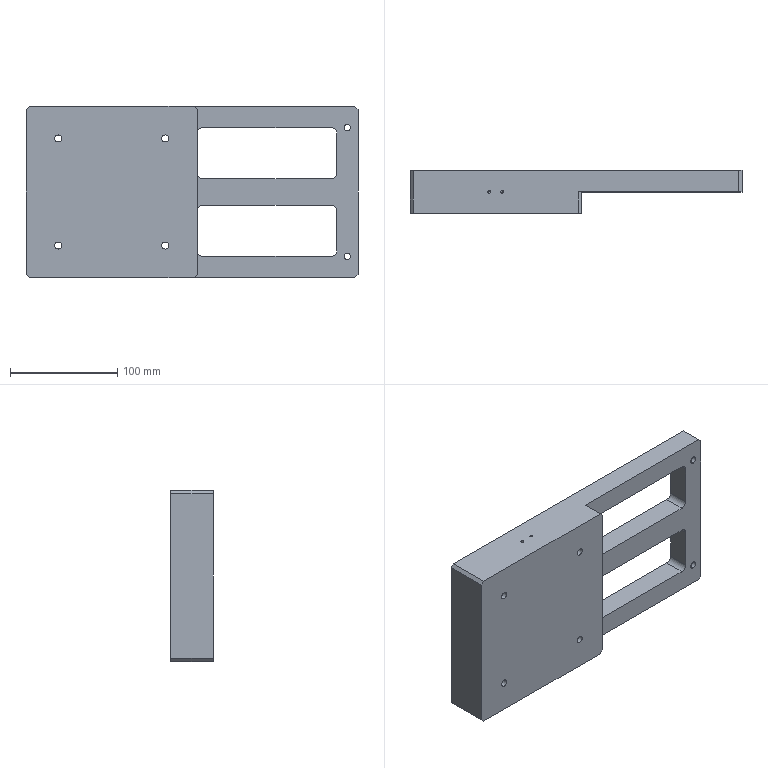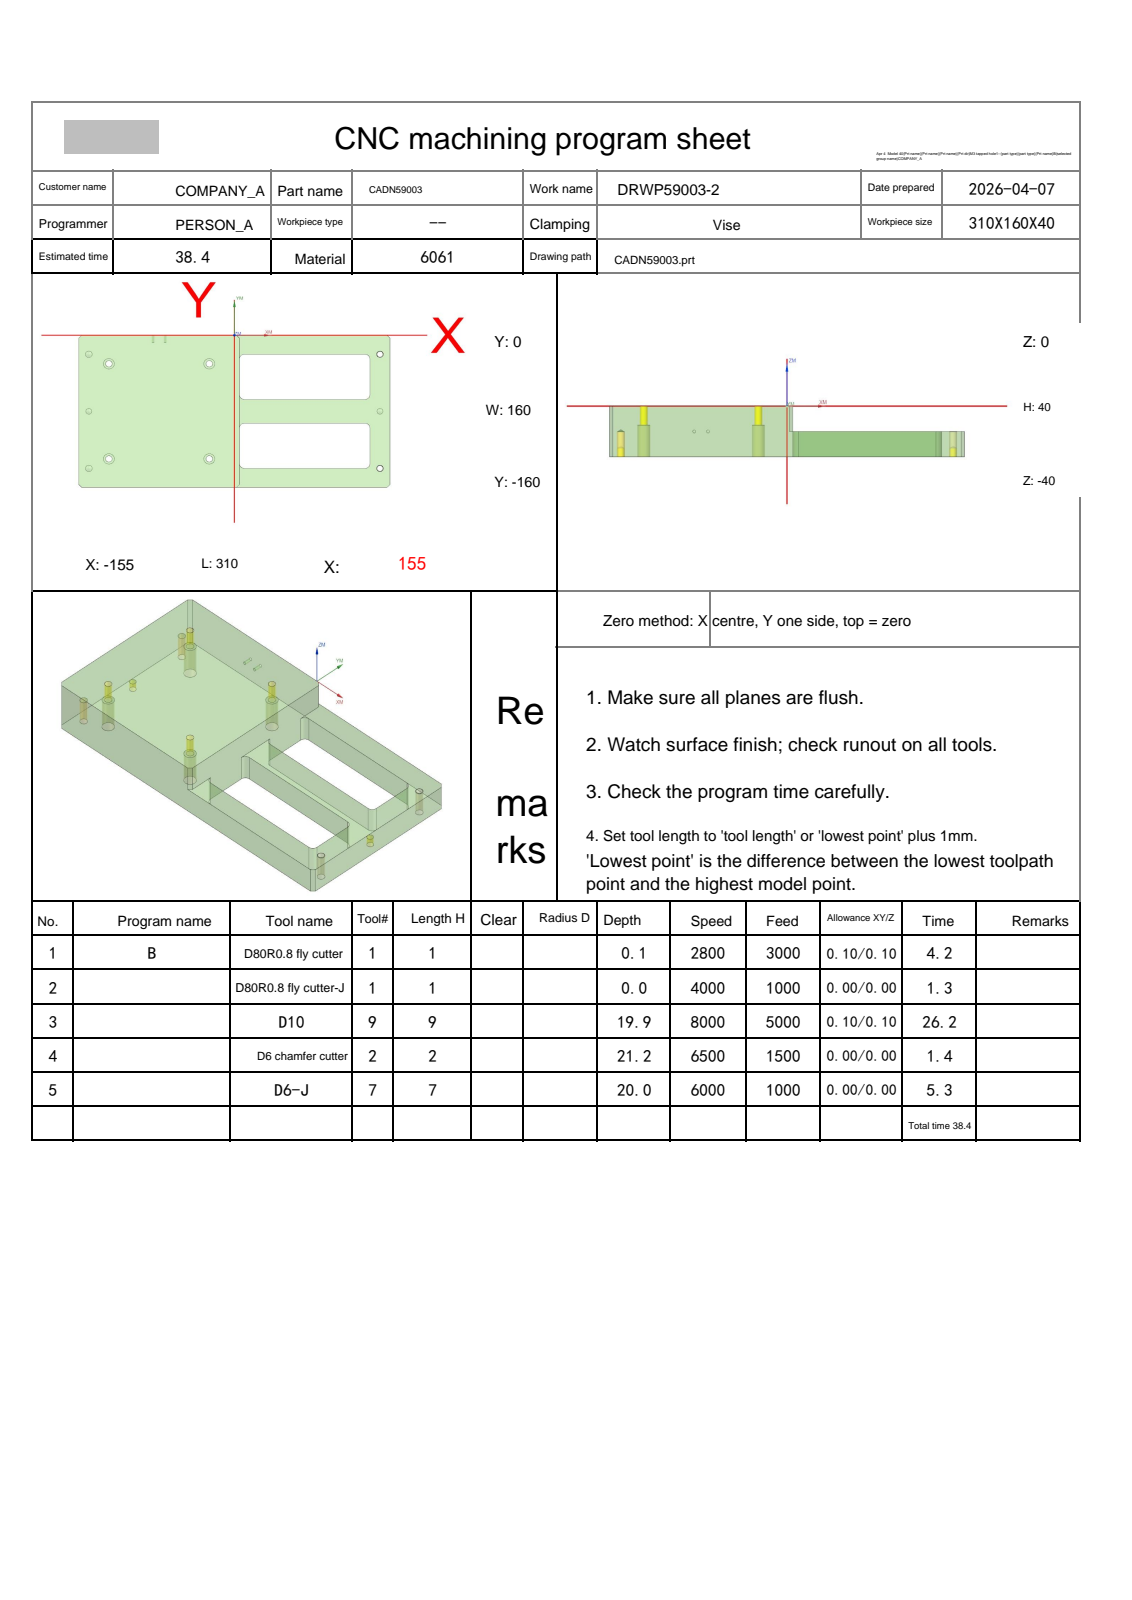NC program | NX | posted by the shop | part box 310 x 40 x 160 mm
Lines 189 to 1206 of 6465:
N3 T09 M06
(D10  D=10. R=0. H=09 ce=0.10 di=0.10)
G00 G90 G54 X157.365 Y8. M03 S8000
G43 H09 Z14.5
M08
Z.915
G01 Z-.585 F5000.
X157.486 Y4.9
G02 X157.6 Y-.877 I-147.386 J-5.788
G01 Y-159.112
G02 X157.521 Y-163.933 I-147.5 J0.0
X156.522 Y-164.9 I-.999 J.033
G01 X153.416
G02 X152.517 Y-164. I.001 J.9
G01 Y-163.97
G03 X152.6 Y-159.112 I-142.417 J4.858
G01 Y-.878
G03 X152.518 Y3.934 I-142.5 J-.01
X151.519 Y4.9 I-.999 J-.034
G01 X145.911
G03 X145.012 Y4. I.001 J-.9
G01 X145.013 Y3.968
G02 X145.1 Y-.878 I-134.913 J-4.856
G01 Y-159.112
G02 X145.014 Y-163.936 I-135. J0.0
X144.015 Y-164.9 I-.999 J.036
G01 X138.406
G02 X137.507 Y-164. I.001 J.9
G01 X137.508 Y-163.967
G03 X137.6 Y-159.112 I-127.408 J4.854
G01 Y-.879
G03 X137.509 Y3.938 I-127.5 J-.009
X136.51 Y4.9 I-.999 J-.038
G01 X130.9
G03 X130.001 Y4. I.001 J-.9
G01 X130.002 Y3.964
G02 X130.1 Y-.879 I-119.902 J-4.852
G01 Y-159.112
G02 X130.003 Y-163.941 I-120. J0.0
X129.004 Y-164.9 I-.999 J.041
G01 X123.394
G02 X122.495 Y-164. I.001 J.9
G01 Y-163.962
G03 X122.6 Y-159.112 I-112.395 J4.85
G01 Y-.88
G03 X122.496 Y3.943 I-112.5 J-.008
X121.497 Y4.9 I-.999 J-.043
G01 X115.886
G03 X114.987 Y4. I.001 J-.9
G01 X114.988 Y3.959
G02 X115.1 Y-.88 I-104.888 J-4.847
G01 Y-159.112
G02 X114.989 Y-163.946 I-105. J0.0
X113.99 Y-164.9 I-.999 J.046
G01 X108.378
G02 X107.479 Y-164. I.001 J.9
G01 X107.48 Y-163.956
G03 X107.6 Y-159.112 I-97.38 J4.844
G01 Y-.881
G03 X107.48 Y3.95 I-97.5 J-.007
X106.481 Y4.9 I-.999 J-.05
G01 X100.868
G03 X99.969 Y4. I.001 J-.9
G01 X99.97 Y3.952
G02 X100.1 Y-.881 I-89.87 J-4.84
G01 Y-159.112
G02 X99.97 Y-163.954 I-90. J0.0
X98.971 Y-164.9 I-.999 J.054
G01 X93.356
G02 X92.457 Y-164. I.001 J.9
G01 X92.458 Y-163.948
G03 X92.6 Y-159.112 I-82.358 J4.836
G01 Y-.882
G03 X92.458 Y3.959 I-82.5 J-.006
X91.46 Y4.9 I-.998 J-.059
G01 X85.842
G03 X84.942 Y4. I.001 J-.9
G01 X84.944 Y3.943
G02 X85.1 Y-.882 I-74.844 J-4.83
G01 Y-159.112
G02 X84.943 Y-163.965 I-75. J0.0
X83.945 Y-164.9 I-.998 J.065
G01 X78.324
G02 X77.425 Y-164. I.001 J.9
G01 X77.427 Y-163.936
G03 X77.6 Y-159.112 I-67.327 J4.824
G01 Y-.883
G03 X77.425 Y3.972 I-67.5 J-.005
X76.428 Y4.9 I-.997 J-.072
G01 X70.803
G03 X69.904 Y4. I.001 J-.9
G01 X69.906 Y3.929
G02 X70.1 Y-.883 I-59.806 J-4.816
G01 Y-159.112
G02 X69.902 Y-163.981 I-60. J0.0
X68.906 Y-164.9 I-.997 J.081
G01 X63.275
G02 X62.376 Y-164. I.001 J.9
G01 X62.38 Y-163.918
G03 X62.6 Y-159.112 I-52.28 J4.806
G01 Y-.884
G03 X62.373 Y3.993 I-52.5 J-.004
X61.377 Y4.9 I-.996 J-.093
G01 X55.627
G03 X54.828 Y4.1 I.001 J-.8
G01 X54.832 Y4.014
G02 X55.1 Y-.884 I-44.732 J-4.901
G01 Y-159.112
G02 X54.833 Y-164.009 I-45. J0.0
X53.839 Y-164.9 I-.994 J.109
G01 X48.073
G02 X47.274 Y-164.1 I.001 J.8
G01 X47.281 Y-163.997
G03 X47.6 Y-159.112 I-37.181 J4.884
G01 Y-.885
G03 X47.276 Y4.031 I-37.5 J-.003
X46.285 Y4.9 I-.991 J-.131
G01 X40.493
G03 X39.693 Y4.1 I.001 J-.8
G01 X39.704 Y3.971
G02 X40.1 Y-.885 I-29.604 J-4.859
G01 Y-159.112
G02 X39.688 Y-164.065 I-30. J0.0
X38.702 Y-164.9 I-.986 J.165
G01 X32.735
G02 X32.035 Y-164.2 I.001 J.7
G01 X32.052 Y-164.047
G03 X32.6 Y-159.112 I-21.952 J4.935
G01 Y-.886
G03 X32.035 Y4.123 I-22.5 J-.002
X31.06 Y4.9 I-.975 J-.223
G01 X24.812
G03 X24.212 Y4.3 I.001 J-.6
X24.246 Y4.101 I.6 J0.0
G02 X25.1 Y-.888 I-14.146 J-4.989
G01 Y-159.112
G02 X24.196 Y-164.242 I-15. J0.0
X23.256 Y-164.9 I-.94 J.342
G01 X15.877
G02 X15.478 Y-164.5 I.001 J.4
X15.585 Y-164.228 I.4 J0.0
G03 X17.6 Y-159.112 I-5.485 J5.115
G01 Y-.888
G03 X15.403 Y4.416 I-7.5 J0.0
G01 X15.143 Y4.676
G03 X14.608 Y4.954 I-.707 J-.707
G01 X5.191 Y6.592
X5.02 Y6.607
G03 X4.02 Y5.607 I0.0 J-1.
X4.312 Y4.9 I1. J0.0
G01 X10.1 Y-.888
Y-159.112
X4.312 Y-164.9
X1.112 Y-168.1
Z.915
G00 Z14.5
X157.365 Y8.
Z.329
G01 Z-1.171
X157.486 Y4.9
G02 X157.6 Y-.877 I-147.386 J-5.788
G01 Y-159.112
G02 X157.521 Y-163.933 I-147.5 J0.0
X156.522 Y-164.9 I-.999 J.033
G01 X153.416
G02 X152.517 Y-164. I.001 J.9
G01 Y-163.97
G03 X152.6 Y-159.112 I-142.417 J4.858
G01 Y-.878
G03 X152.518 Y3.934 I-142.5 J-.01
X151.519 Y4.9 I-.999 J-.034
G01 X145.911
G03 X145.012 Y4. I.001 J-.9
G01 X145.013 Y3.968
G02 X145.1 Y-.878 I-134.913 J-4.856
G01 Y-159.112
G02 X145.014 Y-163.936 I-135. J0.0
X144.015 Y-164.9 I-.999 J.036
G01 X138.406
G02 X137.507 Y-164. I.001 J.9
G01 X137.508 Y-163.967
G03 X137.6 Y-159.112 I-127.408 J4.854
G01 Y-.879
G03 X137.509 Y3.938 I-127.5 J-.009
X136.51 Y4.9 I-.999 J-.038
G01 X130.9
G03 X130.001 Y4. I.001 J-.9
G01 X130.002 Y3.964
G02 X130.1 Y-.879 I-119.902 J-4.852
G01 Y-159.112
G02 X130.003 Y-163.941 I-120. J0.0
X129.004 Y-164.9 I-.999 J.041
G01 X123.394
G02 X122.495 Y-164. I.001 J.9
G01 Y-163.962
G03 X122.6 Y-159.112 I-112.395 J4.85
G01 Y-.88
G03 X122.496 Y3.943 I-112.5 J-.008
X121.497 Y4.9 I-.999 J-.043
G01 X115.886
G03 X114.987 Y4. I.001 J-.9
G01 X114.988 Y3.959
G02 X115.1 Y-.88 I-104.888 J-4.847
G01 Y-159.112
G02 X114.989 Y-163.946 I-105. J0.0
X113.99 Y-164.9 I-.999 J.046
G01 X108.378
G02 X107.479 Y-164. I.001 J.9
G01 X107.48 Y-163.956
G03 X107.6 Y-159.112 I-97.38 J4.844
G01 Y-.881
G03 X107.48 Y3.95 I-97.5 J-.007
X106.481 Y4.9 I-.999 J-.05
G01 X100.868
G03 X99.969 Y4. I.001 J-.9
G01 X99.97 Y3.952
G02 X100.1 Y-.881 I-89.87 J-4.84
G01 Y-159.112
G02 X99.97 Y-163.954 I-90. J0.0
X98.971 Y-164.9 I-.999 J.054
G01 X93.356
G02 X92.457 Y-164. I.001 J.9
G01 X92.458 Y-163.948
G03 X92.6 Y-159.112 I-82.358 J4.836
G01 Y-.882
G03 X92.458 Y3.959 I-82.5 J-.006
X91.46 Y4.9 I-.998 J-.059
G01 X85.842
G03 X84.942 Y4. I.001 J-.9
G01 X84.944 Y3.943
G02 X85.1 Y-.882 I-74.844 J-4.83
G01 Y-159.112
G02 X84.943 Y-163.965 I-75. J0.0
X83.945 Y-164.9 I-.998 J.065
G01 X78.324
G02 X77.425 Y-164. I.001 J.9
G01 X77.427 Y-163.936
G03 X77.6 Y-159.112 I-67.327 J4.824
G01 Y-.883
G03 X77.425 Y3.972 I-67.5 J-.005
X76.428 Y4.9 I-.997 J-.072
G01 X70.803
G03 X69.904 Y4. I.001 J-.9
G01 X69.906 Y3.929
G02 X70.1 Y-.883 I-59.806 J-4.816
G01 Y-159.112
G02 X69.902 Y-163.981 I-60. J0.0
X68.906 Y-164.9 I-.997 J.081
G01 X63.275
G02 X62.376 Y-164. I.001 J.9
G01 X62.38 Y-163.918
G03 X62.6 Y-159.112 I-52.28 J4.806
G01 Y-.884
G03 X62.373 Y3.993 I-52.5 J-.004
X61.377 Y4.9 I-.996 J-.093
G01 X55.627
G03 X54.828 Y4.1 I.001 J-.8
G01 X54.832 Y4.014
G02 X55.1 Y-.884 I-44.732 J-4.901
G01 Y-159.112
G02 X54.833 Y-164.009 I-45. J0.0
X53.839 Y-164.9 I-.994 J.109
G01 X48.073
G02 X47.274 Y-164.1 I.001 J.8
G01 X47.281 Y-163.997
G03 X47.6 Y-159.112 I-37.181 J4.884
G01 Y-.885
G03 X47.276 Y4.031 I-37.5 J-.003
X46.285 Y4.9 I-.991 J-.131
G01 X40.493
G03 X39.693 Y4.1 I.001 J-.8
G01 X39.704 Y3.971
G02 X40.1 Y-.885 I-29.604 J-4.859
G01 Y-159.112
G02 X39.688 Y-164.065 I-30. J0.0
X38.702 Y-164.9 I-.986 J.165
G01 X32.735
G02 X32.035 Y-164.2 I.001 J.7
G01 X32.052 Y-164.047
G03 X32.6 Y-159.112 I-21.952 J4.935
G01 Y-.886
G03 X32.035 Y4.123 I-22.5 J-.002
X31.06 Y4.9 I-.975 J-.223
G01 X24.812
G03 X24.212 Y4.3 I.001 J-.6
X24.246 Y4.101 I.6 J0.0
G02 X25.1 Y-.888 I-14.146 J-4.989
G01 Y-159.112
G02 X24.196 Y-164.242 I-15. J0.0
X23.256 Y-164.9 I-.94 J.342
G01 X15.877
G02 X15.478 Y-164.5 I.001 J.4
X15.585 Y-164.228 I.4 J0.0
G03 X17.6 Y-159.112 I-5.485 J5.115
G01 Y-.888
G03 X15.403 Y4.416 I-7.5 J0.0
G01 X15.143 Y4.676
G03 X14.608 Y4.954 I-.707 J-.707
G01 X5.191 Y6.592
X5.02 Y6.607
G03 X4.02 Y5.607 I0.0 J-1.
X4.312 Y4.9 I1. J0.0
G01 X10.1 Y-.888
Y-159.112
X4.312 Y-164.9
X1.112 Y-168.1
Z.329
G00 Z14.5
X157.365 Y8.
Z-.256
G01 Z-1.756
X157.486 Y4.9
G02 X157.6 Y-.877 I-147.386 J-5.788
G01 Y-159.112
G02 X157.521 Y-163.933 I-147.5 J0.0
X156.522 Y-164.9 I-.999 J.033
G01 X153.416
G02 X152.517 Y-164. I.001 J.9
G01 Y-163.97
G03 X152.6 Y-159.112 I-142.417 J4.858
G01 Y-.878
G03 X152.518 Y3.934 I-142.5 J-.01
X151.519 Y4.9 I-.999 J-.034
G01 X145.911
G03 X145.012 Y4. I.001 J-.9
G01 X145.013 Y3.968
G02 X145.1 Y-.878 I-134.913 J-4.856
G01 Y-159.112
G02 X145.014 Y-163.936 I-135. J0.0
X144.015 Y-164.9 I-.999 J.036
G01 X138.406
G02 X137.507 Y-164. I.001 J.9
G01 X137.508 Y-163.967
G03 X137.6 Y-159.112 I-127.408 J4.854
G01 Y-.879
G03 X137.509 Y3.938 I-127.5 J-.009
X136.51 Y4.9 I-.999 J-.038
G01 X130.9
G03 X130.001 Y4. I.001 J-.9
G01 X130.002 Y3.964
G02 X130.1 Y-.879 I-119.902 J-4.852
G01 Y-159.112
G02 X130.003 Y-163.941 I-120. J0.0
X129.004 Y-164.9 I-.999 J.041
G01 X123.394
G02 X122.495 Y-164. I.001 J.9
G01 Y-163.962
G03 X122.6 Y-159.112 I-112.395 J4.85
G01 Y-.88
G03 X122.496 Y3.943 I-112.5 J-.008
X121.497 Y4.9 I-.999 J-.043
G01 X115.886
G03 X114.987 Y4. I.001 J-.9
G01 X114.988 Y3.959
G02 X115.1 Y-.88 I-104.888 J-4.847
G01 Y-159.112
G02 X114.989 Y-163.946 I-105. J0.0
X113.99 Y-164.9 I-.999 J.046
G01 X108.378
G02 X107.479 Y-164. I.001 J.9
G01 X107.48 Y-163.956
G03 X107.6 Y-159.112 I-97.38 J4.844
G01 Y-.881
G03 X107.48 Y3.95 I-97.5 J-.007
X106.481 Y4.9 I-.999 J-.05
G01 X100.868
G03 X99.969 Y4. I.001 J-.9
G01 X99.97 Y3.952
G02 X100.1 Y-.881 I-89.87 J-4.84
G01 Y-159.112
G02 X99.97 Y-163.954 I-90. J0.0
X98.971 Y-164.9 I-.999 J.054
G01 X93.356
G02 X92.457 Y-164. I.001 J.9
G01 X92.458 Y-163.948
G03 X92.6 Y-159.112 I-82.358 J4.836
G01 Y-.882
G03 X92.458 Y3.959 I-82.5 J-.006
X91.46 Y4.9 I-.998 J-.059
G01 X85.842
G03 X84.942 Y4. I.001 J-.9
G01 X84.944 Y3.943
G02 X85.1 Y-.882 I-74.844 J-4.83
G01 Y-159.112
G02 X84.943 Y-163.965 I-75. J0.0
X83.945 Y-164.9 I-.998 J.065
G01 X78.324
G02 X77.425 Y-164. I.001 J.9
G01 X77.427 Y-163.936
G03 X77.6 Y-159.112 I-67.327 J4.824
G01 Y-.883
G03 X77.425 Y3.972 I-67.5 J-.005
X76.428 Y4.9 I-.997 J-.072
G01 X70.803
G03 X69.904 Y4. I.001 J-.9
G01 X69.906 Y3.929
G02 X70.1 Y-.883 I-59.806 J-4.816
G01 Y-159.112
G02 X69.902 Y-163.981 I-60. J0.0
X68.906 Y-164.9 I-.997 J.081
G01 X63.275
G02 X62.376 Y-164. I.001 J.9
G01 X62.38 Y-163.918
G03 X62.6 Y-159.112 I-52.28 J4.806
G01 Y-.884
G03 X62.373 Y3.993 I-52.5 J-.004
X61.377 Y4.9 I-.996 J-.093
G01 X55.627
G03 X54.828 Y4.1 I.001 J-.8
G01 X54.832 Y4.014
G02 X55.1 Y-.884 I-44.732 J-4.901
G01 Y-159.112
G02 X54.833 Y-164.009 I-45. J0.0
X53.839 Y-164.9 I-.994 J.109
G01 X48.073
G02 X47.274 Y-164.1 I.001 J.8
G01 X47.281 Y-163.997
G03 X47.6 Y-159.112 I-37.181 J4.884
G01 Y-.885
G03 X47.276 Y4.031 I-37.5 J-.003
X46.285 Y4.9 I-.991 J-.131
G01 X40.493
G03 X39.693 Y4.1 I.001 J-.8
G01 X39.704 Y3.971
G02 X40.1 Y-.885 I-29.604 J-4.859
G01 Y-159.112
G02 X39.688 Y-164.065 I-30. J0.0
X38.702 Y-164.9 I-.986 J.165
G01 X32.735
G02 X32.035 Y-164.2 I.001 J.7
G01 X32.052 Y-164.047
G03 X32.6 Y-159.112 I-21.952 J4.935
G01 Y-.886
G03 X32.035 Y4.123 I-22.5 J-.002
X31.06 Y4.9 I-.975 J-.223
G01 X24.812
G03 X24.212 Y4.3 I.001 J-.6
X24.246 Y4.101 I.6 J0.0
G02 X25.1 Y-.888 I-14.146 J-4.989
G01 Y-159.112
G02 X24.196 Y-164.242 I-15. J0.0
X23.256 Y-164.9 I-.94 J.342
G01 X15.877
G02 X15.478 Y-164.5 I.001 J.4
X15.585 Y-164.228 I.4 J0.0
G03 X17.6 Y-159.112 I-5.485 J5.115
G01 Y-.888
G03 X15.403 Y4.416 I-7.5 J0.0
G01 X15.143 Y4.676
G03 X14.608 Y4.954 I-.707 J-.707
G01 X5.191 Y6.592
X5.02 Y6.607
G03 X4.02 Y5.607 I0.0 J-1.
X4.312 Y4.9 I1. J0.0
G01 X10.1 Y-.888
Y-159.112
X4.312 Y-164.9
X1.112 Y-168.1
Z-.256
G00 Z14.5
X157.365 Y8.
Z-.841
G01 Z-2.341
X157.486 Y4.9
G02 X157.6 Y-.877 I-147.386 J-5.788
G01 Y-159.112
G02 X157.521 Y-163.933 I-147.5 J0.0
X156.522 Y-164.9 I-.999 J.033
G01 X153.416
G02 X152.517 Y-164. I.001 J.9
G01 Y-163.97
G03 X152.6 Y-159.112 I-142.417 J4.858
G01 Y-.878
G03 X152.518 Y3.934 I-142.5 J-.01
X151.519 Y4.9 I-.999 J-.034
G01 X145.911
G03 X145.012 Y4. I.001 J-.9
G01 X145.013 Y3.968
G02 X145.1 Y-.878 I-134.913 J-4.856
G01 Y-159.112
G02 X145.014 Y-163.936 I-135. J0.0
X144.015 Y-164.9 I-.999 J.036
G01 X138.406
G02 X137.507 Y-164. I.001 J.9
G01 X137.508 Y-163.967
G03 X137.6 Y-159.112 I-127.408 J4.854
G01 Y-.879
G03 X137.509 Y3.938 I-127.5 J-.009
X136.51 Y4.9 I-.999 J-.038
G01 X130.9
G03 X130.001 Y4. I.001 J-.9
G01 X130.002 Y3.964
G02 X130.1 Y-.879 I-119.902 J-4.852
G01 Y-159.112
G02 X130.003 Y-163.941 I-120. J0.0
X129.004 Y-164.9 I-.999 J.041
G01 X123.394
G02 X122.495 Y-164. I.001 J.9
G01 Y-163.962
G03 X122.6 Y-159.112 I-112.395 J4.85
G01 Y-.88
G03 X122.496 Y3.943 I-112.5 J-.008
X121.497 Y4.9 I-.999 J-.043
G01 X115.886
G03 X114.987 Y4. I.001 J-.9
G01 X114.988 Y3.959
G02 X115.1 Y-.88 I-104.888 J-4.847
G01 Y-159.112
G02 X114.989 Y-163.946 I-105. J0.0
X113.99 Y-164.9 I-.999 J.046
G01 X108.378
G02 X107.479 Y-164. I.001 J.9
G01 X107.48 Y-163.956
G03 X107.6 Y-159.112 I-97.38 J4.844
G01 Y-.881
G03 X107.48 Y3.95 I-97.5 J-.007
X106.481 Y4.9 I-.999 J-.05
G01 X100.868
G03 X99.969 Y4. I.001 J-.9
G01 X99.97 Y3.952
G02 X100.1 Y-.881 I-89.87 J-4.84
G01 Y-159.112
G02 X99.97 Y-163.954 I-90. J0.0
X98.971 Y-164.9 I-.999 J.054
G01 X93.356
G02 X92.457 Y-164. I.001 J.9
G01 X92.458 Y-163.948
G03 X92.6 Y-159.112 I-82.358 J4.836
G01 Y-.882
G03 X92.458 Y3.959 I-82.5 J-.006
X91.46 Y4.9 I-.998 J-.059
G01 X85.842
G03 X84.942 Y4. I.001 J-.9
G01 X84.944 Y3.943
G02 X85.1 Y-.882 I-74.844 J-4.83
G01 Y-159.112
G02 X84.943 Y-163.965 I-75. J0.0
X83.945 Y-164.9 I-.998 J.065
G01 X78.324
G02 X77.425 Y-164. I.001 J.9
G01 X77.427 Y-163.936
G03 X77.6 Y-159.112 I-67.327 J4.824
G01 Y-.883
G03 X77.425 Y3.972 I-67.5 J-.005
X76.428 Y4.9 I-.997 J-.072
G01 X70.803
G03 X69.904 Y4. I.001 J-.9
G01 X69.906 Y3.929
G02 X70.1 Y-.883 I-59.806 J-4.816
G01 Y-159.112
G02 X69.902 Y-163.981 I-60. J0.0
X68.906 Y-164.9 I-.997 J.081
G01 X63.275
G02 X62.376 Y-164. I.001 J.9
G01 X62.38 Y-163.918
G03 X62.6 Y-159.112 I-52.28 J4.806
G01 Y-.884
G03 X62.373 Y3.993 I-52.5 J-.004
X61.377 Y4.9 I-.996 J-.093
G01 X55.627
G03 X54.828 Y4.1 I.001 J-.8
G01 X54.832 Y4.014
G02 X55.1 Y-.884 I-44.732 J-4.901
G01 Y-159.112
G02 X54.833 Y-164.009 I-45. J0.0
X53.839 Y-164.9 I-.994 J.109
G01 X48.073
G02 X47.274 Y-164.1 I.001 J.8
G01 X47.281 Y-163.997
G03 X47.6 Y-159.112 I-37.181 J4.884
G01 Y-.885
G03 X47.276 Y4.031 I-37.5 J-.003
X46.285 Y4.9 I-.991 J-.131
G01 X40.493
G03 X39.693 Y4.1 I.001 J-.8
G01 X39.704 Y3.971
G02 X40.1 Y-.885 I-29.604 J-4.859
G01 Y-159.112
G02 X39.688 Y-164.065 I-30. J0.0
X38.702 Y-164.9 I-.986 J.165
G01 X32.735
G02 X32.035 Y-164.2 I.001 J.7
G01 X32.052 Y-164.047
G03 X32.6 Y-159.112 I-21.952 J4.935
G01 Y-.886
G03 X32.035 Y4.123 I-22.5 J-.002
X31.06 Y4.9 I-.975 J-.223
G01 X24.812
G03 X24.212 Y4.3 I.001 J-.6
X24.246 Y4.101 I.6 J0.0
G02 X25.1 Y-.888 I-14.146 J-4.989
G01 Y-159.112
G02 X24.196 Y-164.242 I-15. J0.0
X23.256 Y-164.9 I-.94 J.342
G01 X15.877
G02 X15.478 Y-164.5 I.001 J.4
X15.585 Y-164.228 I.4 J0.0
G03 X17.6 Y-159.112 I-5.485 J5.115
G01 Y-.888
G03 X15.403 Y4.416 I-7.5 J0.0
G01 X15.143 Y4.676
G03 X14.608 Y4.954 I-.707 J-.707
G01 X5.191 Y6.592
X5.02 Y6.607
G03 X4.02 Y5.607 I0.0 J-1.
X4.312 Y4.9 I1. J0.0
G01 X10.1 Y-.888
Y-159.112
X4.312 Y-164.9
X1.112 Y-168.1
Z-.841
G00 Z14.5
X157.365 Y8.
Z-1.426
G01 Z-2.926
X157.486 Y4.9
G02 X157.6 Y-.877 I-147.386 J-5.788
G01 Y-159.112
G02 X157.521 Y-163.933 I-147.5 J0.0
X156.522 Y-164.9 I-.999 J.033
G01 X153.416
G02 X152.517 Y-164. I.001 J.9
G01 Y-163.97
G03 X152.6 Y-159.112 I-142.417 J4.858
G01 Y-.878
G03 X152.518 Y3.934 I-142.5 J-.01
X151.519 Y4.9 I-.999 J-.034
G01 X145.911
G03 X145.012 Y4. I.001 J-.9
G01 X145.013 Y3.968
G02 X145.1 Y-.878 I-134.913 J-4.856
G01 Y-159.112
G02 X145.014 Y-163.936 I-135. J0.0
X144.015 Y-164.9 I-.999 J.036
G01 X138.406
G02 X137.507 Y-164. I.001 J.9
G01 X137.508 Y-163.967
G03 X137.6 Y-159.112 I-127.408 J4.854
G01 Y-.879
G03 X137.509 Y3.938 I-127.5 J-.009
X136.51 Y4.9 I-.999 J-.038
G01 X130.9
G03 X130.001 Y4. I.001 J-.9
G01 X130.002 Y3.964
G02 X130.1 Y-.879 I-119.902 J-4.852
G01 Y-159.112
G02 X130.003 Y-163.941 I-120. J0.0
X129.004 Y-164.9 I-.999 J.041
G01 X123.394
G02 X122.495 Y-164. I.001 J.9
G01 Y-163.962
G03 X122.6 Y-159.112 I-112.395 J4.85
G01 Y-.88
G03 X122.496 Y3.943 I-112.5 J-.008
X121.497 Y4.9 I-.999 J-.043
G01 X115.886
G03 X114.987 Y4. I.001 J-.9
G01 X114.988 Y3.959
G02 X115.1 Y-.88 I-104.888 J-4.847
G01 Y-159.112
G02 X114.989 Y-163.946 I-105. J0.0
X113.99 Y-164.9 I-.999 J.046
G01 X108.378
G02 X107.479 Y-164. I.001 J.9
G01 X107.48 Y-163.956
G03 X107.6 Y-159.112 I-97.38 J4.844
G01 Y-.881
G03 X107.48 Y3.95 I-97.5 J-.007
X106.481 Y4.9 I-.999 J-.05
G01 X100.868
G03 X99.969 Y4. I.001 J-.9
G01 X99.97 Y3.952
G02 X100.1 Y-.881 I-89.87 J-4.84
G01 Y-159.112
G02 X99.97 Y-163.954 I-90. J0.0
X98.971 Y-164.9 I-.999 J.054
G01 X93.356
G02 X92.457 Y-164. I.001 J.9
G01 X92.458 Y-163.948
G03 X92.6 Y-159.112 I-82.358 J4.836
G01 Y-.882
G03 X92.458 Y3.959 I-82.5 J-.006
X91.46 Y4.9 I-.998 J-.059
G01 X85.842
G03 X84.942 Y4. I.001 J-.9
G01 X84.944 Y3.943
G02 X85.1 Y-.882 I-74.844 J-4.83
G01 Y-159.112
G02 X84.943 Y-163.965 I-75. J0.0
X83.945 Y-164.9 I-.998 J.065
G01 X78.324
G02 X77.425 Y-164. I.001 J.9
G01 X77.427 Y-163.936
G03 X77.6 Y-159.112 I-67.327 J4.824
G01 Y-.883
G03 X77.425 Y3.972 I-67.5 J-.005
X76.428 Y4.9 I-.997 J-.072
G01 X70.803
G03 X69.904 Y4. I.001 J-.9
G01 X69.906 Y3.929
G02 X70.1 Y-.883 I-59.806 J-4.816
G01 Y-159.112
G02 X69.902 Y-163.981 I-60. J0.0
X68.906 Y-164.9 I-.997 J.081
G01 X63.275
G02 X62.376 Y-164. I.001 J.9
G01 X62.38 Y-163.918
G03 X62.6 Y-159.112 I-52.28 J4.806
G01 Y-.884
G03 X62.373 Y3.993 I-52.5 J-.004
X61.377 Y4.9 I-.996 J-.093
G01 X55.627
G03 X54.828 Y4.1 I.001 J-.8
G01 X54.832 Y4.014
G02 X55.1 Y-.884 I-44.732 J-4.901
G01 Y-159.112
G02 X54.833 Y-164.009 I-45. J0.0
X53.839 Y-164.9 I-.994 J.109
G01 X48.073
G02 X47.274 Y-164.1 I.001 J.8
G01 X47.281 Y-163.997
G03 X47.6 Y-159.112 I-37.181 J4.884
G01 Y-.885
G03 X47.276 Y4.031 I-37.5 J-.003
X46.285 Y4.9 I-.991 J-.131
G01 X40.493
G03 X39.693 Y4.1 I.001 J-.8
G01 X39.704 Y3.971
G02 X40.1 Y-.885 I-29.604 J-4.859
G01 Y-159.112
G02 X39.688 Y-164.065 I-30. J0.0
X38.702 Y-164.9 I-.986 J.165
G01 X32.735
G02 X32.035 Y-164.2 I.001 J.7
G01 X32.052 Y-164.047
G03 X32.6 Y-159.112 I-21.952 J4.935
G01 Y-.886
G03 X32.035 Y4.123 I-22.5 J-.002
X31.06 Y4.9 I-.975 J-.223
G01 X24.812
G03 X24.212 Y4.3 I.001 J-.6
X24.246 Y4.101 I.6 J0.0
G02 X25.1 Y-.888 I-14.146 J-4.989
G01 Y-159.112
G02 X24.196 Y-164.242 I-15. J0.0
X23.256 Y-164.9 I-.94 J.342
G01 X15.877
G02 X15.478 Y-164.5 I.001 J.4
X15.585 Y-164.228 I.4 J0.0
G03 X17.6 Y-159.112 I-5.485 J5.115
G01 Y-.888
G03 X15.403 Y4.416 I-7.5 J0.0
G01 X15.143 Y4.676
G03 X14.608 Y4.954 I-.707 J-.707
G01 X5.191 Y6.592
X5.02 Y6.607
G03 X4.02 Y5.607 I0.0 J-1.
X4.312 Y4.9 I1. J0.0
G01 X10.1 Y-.888
Y-159.112
X4.312 Y-164.9
X1.112 Y-168.1
Z-1.426
G00 Z14.5
X157.365 Y8.
Z-2.012
G01 Z-3.512
X157.486 Y4.9
G02 X157.6 Y-.877 I-147.386 J-5.788
G01 Y-159.112
G02 X157.521 Y-163.933 I-147.5 J0.0
X156.522 Y-164.9 I-.999 J.033
G01 X153.416
G02 X152.517 Y-164. I.001 J.9
G01 Y-163.97
G03 X152.6 Y-159.112 I-142.417 J4.858
G01 Y-.878
G03 X152.518 Y3.934 I-142.5 J-.01
X151.519 Y4.9 I-.999 J-.034
G01 X145.911
G03 X145.012 Y4. I.001 J-.9
G01 X145.013 Y3.968
G02 X145.1 Y-.878 I-134.913 J-4.856
G01 Y-159.112
G02 X145.014 Y-163.936 I-135. J0.0
X144.015 Y-164.9 I-.999 J.036
G01 X138.406
G02 X137.507 Y-164. I.001 J.9
G01 X137.508 Y-163.967
G03 X137.6 Y-159.112 I-127.408 J4.854
G01 Y-.879
G03 X137.509 Y3.938 I-127.5 J-.009
X136.51 Y4.9 I-.999 J-.038
G01 X130.9
G03 X130.001 Y4. I.001 J-.9
G01 X130.002 Y3.964
G02 X130.1 Y-.879 I-119.902 J-4.852
G01 Y-159.112
G02 X130.003 Y-163.941 I-120. J0.0
X129.004 Y-164.9 I-.999 J.041
G01 X123.394
G02 X122.495 Y-164. I.001 J.9
G01 Y-163.962
G03 X122.6 Y-159.112 I-112.395 J4.85
G01 Y-.88
G03 X122.496 Y3.943 I-112.5 J-.008
X121.497 Y4.9 I-.999 J-.043
G01 X115.886
G03 X114.987 Y4. I.001 J-.9
G01 X114.988 Y3.959
G02 X115.1 Y-.88 I-104.888 J-4.847
G01 Y-159.112
G02 X114.989 Y-163.946 I-105. J0.0
X113.99 Y-164.9 I-.999 J.046
G01 X108.378
G02 X107.479 Y-164. I.001 J.9
G01 X107.48 Y-163.956
G03 X107.6 Y-159.112 I-97.38 J4.844
G01 Y-.881
G03 X107.48 Y3.95 I-97.5 J-.007
X106.481 Y4.9 I-.999 J-.05
G01 X100.868
G03 X99.969 Y4. I.001 J-.9
G01 X99.97 Y3.952
G02 X100.1 Y-.881 I-89.87 J-4.84
G01 Y-159.112
G02 X99.97 Y-163.954 I-90. J0.0
X98.971 Y-164.9 I-.999 J.054
G01 X93.356
G02 X92.457 Y-164. I.001 J.9
G01 X92.458 Y-163.948
G03 X92.6 Y-159.112 I-82.358 J4.836
G01 Y-.882
G03 X92.458 Y3.959 I-82.5 J-.006
X91.46 Y4.9 I-.998 J-.059
G01 X85.842
G03 X84.942 Y4. I.001 J-.9
G01 X84.944 Y3.943
G02 X85.1 Y-.882 I-74.844 J-4.83
G01 Y-159.112
G02 X84.943 Y-163.965 I-75. J0.0
X83.945 Y-164.9 I-.998 J.065
G01 X78.324
G02 X77.425 Y-164. I.001 J.9
G01 X77.427 Y-163.936
G03 X77.6 Y-159.112 I-67.327 J4.824
G01 Y-.883
G03 X77.425 Y3.972 I-67.5 J-.005
X76.428 Y4.9 I-.997 J-.072
G01 X70.803
G03 X69.904 Y4. I.001 J-.9
G01 X69.906 Y3.929
G02 X70.1 Y-.883 I-59.806 J-4.816
G01 Y-159.112
G02 X69.902 Y-163.981 I-60. J0.0
X68.906 Y-164.9 I-.997 J.081
G01 X63.275
G02 X62.376 Y-164. I.001 J.9
G01 X62.38 Y-163.918
G03 X62.6 Y-159.112 I-52.28 J4.806
G01 Y-.884
G03 X62.373 Y3.993 I-52.5 J-.004
X61.377 Y4.9 I-.996 J-.093
G01 X55.627
G03 X54.828 Y4.1 I.001 J-.8
G01 X54.832 Y4.014
G02 X55.1 Y-.884 I-44.732 J-4.901
G01 Y-159.112
G02 X54.833 Y-164.009 I-45. J0.0
X53.839 Y-164.9 I-.994 J.109
G01 X48.073
G02 X47.274 Y-164.1 I.001 J.8
G01 X47.281 Y-163.997
G03 X47.6 Y-159.112 I-37.181 J4.884
G01 Y-.885
G03 X47.276 Y4.031 I-37.5 J-.003
X46.285 Y4.9 I-.991 J-.131
G01 X40.493
G03 X39.693 Y4.1 I.001 J-.8
G01 X39.704 Y3.971
G02 X40.1 Y-.885 I-29.604 J-4.859
G01 Y-159.112
G02 X39.688 Y-164.065 I-30. J0.0
X38.702 Y-164.9 I-.986 J.165
G01 X32.735
G02 X32.035 Y-164.2 I.001 J.7
G01 X32.052 Y-164.047
G03 X32.6 Y-159.112 I-21.952 J4.935
G01 Y-.886
G03 X32.035 Y4.123 I-22.5 J-.002
X31.06 Y4.9 I-.975 J-.223
G01 X24.812
G03 X24.212 Y4.3 I.001 J-.6
X24.246 Y4.101 I.6 J0.0
G02 X25.1 Y-.888 I-14.146 J-4.989
G01 Y-159.112
G02 X24.196 Y-164.242 I-15. J0.0
X23.256 Y-164.9 I-.94 J.342
G01 X15.877
G02 X15.478 Y-164.5 I.001 J.4
X15.585 Y-164.228 I.4 J0.0
G03 X17.6 Y-159.112 I-5.485 J5.115
G01 Y-.888
G03 X15.403 Y4.416 I-7.5 J0.0
G01 X15.143 Y4.676
G03 X14.608 Y4.954 I-.707 J-.707
G01 X5.191 Y6.592
X5.02 Y6.607
G03 X4.02 Y5.607 I0.0 J-1.
X4.312 Y4.9 I1. J0.0
G01 X10.1 Y-.888
Y-159.112
X4.312 Y-164.9
X1.112 Y-168.1
Z-2.012
G00 Z14.5
X157.365 Y8.
Z-2.597
G01 Z-4.097
X157.486 Y4.9
G02 X157.6 Y-.877 I-147.386 J-5.788
G01 Y-159.112
G02 X157.521 Y-163.933 I-147.5 J0.0
X156.522 Y-164.9 I-.999 J.033
G01 X153.416
G02 X152.517 Y-164. I.001 J.9
G01 Y-163.97
G03 X152.6 Y-159.112 I-142.417 J4.858
G01 Y-.878
G03 X152.518 Y3.934 I-142.5 J-.01
X151.519 Y4.9 I-.999 J-.034
G01 X145.911
G03 X145.012 Y4. I.001 J-.9
G01 X145.013 Y3.968
G02 X145.1 Y-.878 I-134.913 J-4.856
G01 Y-159.112
G02 X145.014 Y-163.936 I-135. J0.0
X144.015 Y-164.9 I-.999 J.036
G01 X138.406
G02 X137.507 Y-164. I.001 J.9
G01 X137.508 Y-163.967
G03 X137.6 Y-159.112 I-127.408 J4.854
G01 Y-.879
G03 X137.509 Y3.938 I-127.5 J-.009
X136.51 Y4.9 I-.999 J-.038
G01 X130.9
G03 X130.001 Y4. I.001 J-.9
G01 X130.002 Y3.964
G02 X130.1 Y-.879 I-119.902 J-4.852
G01 Y-159.112
G02 X130.003 Y-163.941 I-120. J0.0
X129.004 Y-164.9 I-.999 J.041
G01 X123.394
G02 X122.495 Y-164. I.001 J.9
G01 Y-163.962
G03 X122.6 Y-159.112 I-112.395 J4.85
G01 Y-.88
G03 X122.496 Y3.943 I-112.5 J-.008
X121.497 Y4.9 I-.999 J-.043
G01 X115.886
G03 X114.987 Y4. I.001 J-.9
G01 X114.988 Y3.959
G02 X115.1 Y-.88 I-104.888 J-4.847
G01 Y-159.112
G02 X114.989 Y-163.946 I-105. J0.0
X113.99 Y-164.9 I-.999 J.046
G01 X108.378
G02 X107.479 Y-164. I.001 J.9
G01 X107.48 Y-163.956
G03 X107.6 Y-159.112 I-97.38 J4.844
G01 Y-.881
G03 X107.48 Y3.95 I-97.5 J-.007
X106.481 Y4.9 I-.999 J-.05
G01 X100.868
G03 X99.969 Y4. I.001 J-.9
G01 X99.97 Y3.952
G02 X100.1 Y-.881 I-89.87 J-4.84
G01 Y-159.112
G02 X99.97 Y-163.954 I-90. J0.0
X98.971 Y-164.9 I-.999 J.054
G01 X93.356
G02 X92.457 Y-164. I.001 J.9
G01 X92.458 Y-163.948
G03 X92.6 Y-159.112 I-82.358 J4.836
G01 Y-.882
G03 X92.458 Y3.959 I-82.5 J-.006
X91.46 Y4.9 I-.998 J-.059
G01 X85.842
G03 X84.942 Y4. I.001 J-.9
G01 X84.944 Y3.943
G02 X85.1 Y-.882 I-74.844 J-4.83
G01 Y-159.112
G02 X84.943 Y-163.965 I-75. J0.0
X83.945 Y-164.9 I-.998 J.065
G01 X78.324
G02 X77.425 Y-164. I.001 J.9
G01 X77.427 Y-163.936
G03 X77.6 Y-159.112 I-67.327 J4.824
G01 Y-.883
G03 X77.425 Y3.972 I-67.5 J-.005
X76.428 Y4.9 I-.997 J-.072
G01 X70.803
G03 X69.904 Y4. I.001 J-.9
G01 X69.906 Y3.929
G02 X70.1 Y-.883 I-59.806 J-4.816
G01 Y-159.112
G02 X69.902 Y-163.981 I-60. J0.0
X68.906 Y-164.9 I-.997 J.081
G01 X63.275
G02 X62.376 Y-164. I.001 J.9
G01 X62.38 Y-163.918
G03 X62.6 Y-159.112 I-52.28 J4.806
G01 Y-.884
G03 X62.373 Y3.993 I-52.5 J-.004
X61.377 Y4.9 I-.996 J-.093
G01 X55.627
G03 X54.828 Y4.1 I.001 J-.8
G01 X54.832 Y4.014